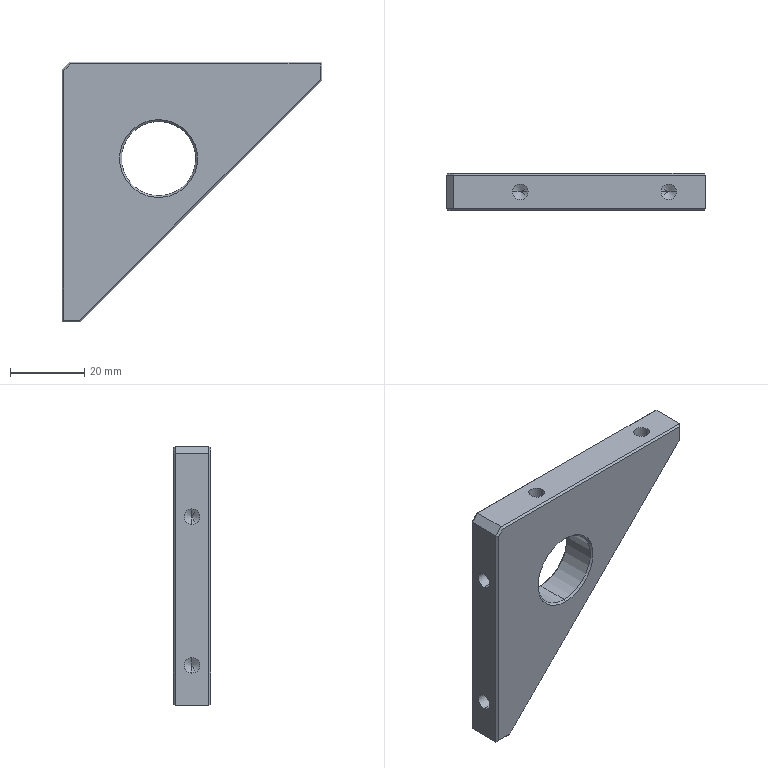Part | SolidWorks | features Chamfer 2, HoleWzd 2, Cut 1, Extrusion 1 | 1 solid | 42 faces | box 70 x 10 x 70 mm | volume 23927 mm3 | plane 20 | cone 12 | cylinder 10 | commonest cylinder face diameters 4.2 x8 20 x2
STEP:
#1=CARTESIAN_POINT('',(26.,4.5,-36.));
#2=VERTEX_POINT('',#1);
#3=CARTESIAN_POINT('',(26.,4.5,-16.));
#4=VERTEX_POINT('',#3);
#5=CARTESIAN_POINT('',(26.,4.5,-26.));
#6=DIRECTION('',(0.,1.,0.));
#7=DIRECTION('',(0.,0.,-1.));
#8=AXIS2_PLACEMENT_3D('',#5,#6,#7);
#9=CIRCLE('',#8,10.);
#10=EDGE_CURVE('',#2,#4,#9,.T.);
#11=ORIENTED_EDGE('',*,*,#10,.F.);
#12=CARTESIAN_POINT('',(26.,5.,-36.5));
#13=VERTEX_POINT('',#12);
#14=CARTESIAN_POINT('',(26.,5.,-36.5));
#15=DIRECTION('',(0.,0.7071,-0.7071));
#16=VECTOR('',#15,1000.);
#17=LINE('',#14,#16);
#18=EDGE_CURVE('',#2,#13,#17,.T.);
#19=ORIENTED_EDGE('',*,*,#18,.T.);
#20=CARTESIAN_POINT('',(26.,5.,-15.5));
#21=VERTEX_POINT('',#20);
#22=CARTESIAN_POINT('',(26.,5.,-26.));
#23=DIRECTION('',(0.,-1.,0.));
#24=DIRECTION('',(0.,0.,-1.));
#25=AXIS2_PLACEMENT_3D('',#22,#23,#24);
#26=CIRCLE('',#25,10.5);
#27=EDGE_CURVE('',#21,#13,#26,.T.);
#28=ORIENTED_EDGE('',*,*,#27,.F.);
#29=CARTESIAN_POINT('',(26.,5.,-15.5));
#30=DIRECTION('',(0.,0.7071,0.7071));
#31=VECTOR('',#30,1000.);
#32=LINE('',#29,#31);
#33=EDGE_CURVE('',#4,#21,#32,.T.);
#34=ORIENTED_EDGE('',*,*,#33,.F.);
#35=EDGE_LOOP('',(#11,#19,#28,#34));
#36=FACE_OUTER_BOUND('',#35,.T.);
#37=CARTESIAN_POINT('',(26.,5.,-26.));
#38=DIRECTION('',(0.,1.,0.));
#39=DIRECTION('',(0.,0.,1.));
#40=AXIS2_PLACEMENT_3D('',#37,#38,#39);
#41=CONICAL_SURFACE('',#40,10.5,0.7854);
#42=ADVANCED_FACE('',(#36),#41,.F.);
#43=CARTESIAN_POINT('',(26.,-4.5,-16.));
#44=VERTEX_POINT('',#43);
#45=CARTESIAN_POINT('',(26.,-4.5,-36.));
#46=VERTEX_POINT('',#45);
#47=CARTESIAN_POINT('',(26.,-4.5,-26.));
#48=DIRECTION('',(0.,-1.,0.));
#49=DIRECTION('',(0.,0.,-1.));
#50=AXIS2_PLACEMENT_3D('',#47,#48,#49);
#51=CIRCLE('',#50,10.);
#52=EDGE_CURVE('',#44,#46,#51,.T.);
#53=ORIENTED_EDGE('',*,*,#52,.F.);
#54=CARTESIAN_POINT('',(26.,-5.,-15.5));
#55=VERTEX_POINT('',#54);
#56=CARTESIAN_POINT('',(26.,-4.5,-16.));
#57=DIRECTION('',(0.,-0.7071,0.7071));
#58=VECTOR('',#57,1000.);
#59=LINE('',#56,#58);
#60=EDGE_CURVE('',#44,#55,#59,.T.);
#61=ORIENTED_EDGE('',*,*,#60,.T.);
#62=CARTESIAN_POINT('',(26.,-5.,-36.5));
#63=VERTEX_POINT('',#62);
#64=CARTESIAN_POINT('',(26.,-5.,-26.));
#65=DIRECTION('',(0.,1.,0.));
#66=DIRECTION('',(0.,0.,-1.));
#67=AXIS2_PLACEMENT_3D('',#64,#65,#66);
#68=CIRCLE('',#67,10.5);
#69=EDGE_CURVE('',#63,#55,#68,.T.);
#70=ORIENTED_EDGE('',*,*,#69,.F.);
#71=CARTESIAN_POINT('',(26.,-4.5,-36.));
#72=DIRECTION('',(0.,-0.7071,-0.7071));
#73=VECTOR('',#72,1000.);
#74=LINE('',#71,#73);
#75=EDGE_CURVE('',#46,#63,#74,.T.);
#76=ORIENTED_EDGE('',*,*,#75,.F.);
#77=EDGE_LOOP('',(#53,#61,#70,#76));
#78=FACE_OUTER_BOUND('',#77,.T.);
#79=CARTESIAN_POINT('',(26.,-4.5,-26.));
#80=DIRECTION('',(0.,-1.,0.));
#81=DIRECTION('',(0.,0.,-1.));
#82=AXIS2_PLACEMENT_3D('',#79,#80,#81);
#83=CONICAL_SURFACE('',#82,10.,0.7854);
#84=ADVANCED_FACE('',(#78),#83,.F.);
#85=ORIENTED_EDGE('',*,*,#10,.T.);
#86=CARTESIAN_POINT('',(26.,5.,-16.));
#87=DIRECTION('',(0.,-1.,0.));
#88=VECTOR('',#87,1000.);
#89=LINE('',#86,#88);
#90=EDGE_CURVE('',#4,#44,#89,.T.);
#91=ORIENTED_EDGE('',*,*,#90,.T.);
#92=ORIENTED_EDGE('',*,*,#52,.T.);
#93=CARTESIAN_POINT('',(26.,5.,-36.));
#94=DIRECTION('',(0.,-1.,0.));
#95=VECTOR('',#94,1000.);
#96=LINE('',#93,#95);
#97=EDGE_CURVE('',#2,#46,#96,.T.);
#98=ORIENTED_EDGE('',*,*,#97,.F.);
#99=EDGE_LOOP('',(#85,#91,#92,#98));
#100=FACE_OUTER_BOUND('',#99,.T.);
#101=CARTESIAN_POINT('',(26.,5.,-26.));
#102=DIRECTION('',(0.,-1.,0.));
#103=DIRECTION('',(0.,0.,-1.));
#104=AXIS2_PLACEMENT_3D('',#101,#102,#103);
#105=CYLINDRICAL_SURFACE('',#104,10.);
#106=ADVANCED_FACE('',(#100),#105,.F.);
#107=CARTESIAN_POINT('',(12.4,0.,-21.154));
#108=VERTEX_POINT('',#107);
#109=CARTESIAN_POINT('',(12.4,0.,-16.954));
#110=VERTEX_POINT('',#109);
#111=CARTESIAN_POINT('',(12.4,0.,-19.054));
#112=DIRECTION('',(-1.,0.,0.));
#113=DIRECTION('',(0.,0.,1.));
#114=AXIS2_PLACEMENT_3D('',#111,#112,#113);
#115=CIRCLE('',#114,2.1);
#116=EDGE_CURVE('',#108,#110,#115,.T.);
#117=ORIENTED_EDGE('',*,*,#116,.F.);
#118=CARTESIAN_POINT('',(0.,0.,-21.154));
#119=VERTEX_POINT('',#118);
#120=CARTESIAN_POINT('',(0.,0.,-21.154));
#121=DIRECTION('',(-1.,0.,0.));
#122=VECTOR('',#121,1000.);
#123=LINE('',#120,#122);
#124=EDGE_CURVE('',#108,#119,#123,.T.);
#125=ORIENTED_EDGE('',*,*,#124,.T.);
#126=CARTESIAN_POINT('',(0.,0.,-16.954));
#127=VERTEX_POINT('',#126);
#128=CARTESIAN_POINT('',(0.,0.,-19.054));
#129=DIRECTION('',(-1.,0.,0.));
#130=DIRECTION('',(0.,0.,1.));
#131=AXIS2_PLACEMENT_3D('',#128,#129,#130);
#132=CIRCLE('',#131,2.1);
#133=EDGE_CURVE('',#119,#127,#132,.T.);
#134=ORIENTED_EDGE('',*,*,#133,.T.);
#135=CARTESIAN_POINT('',(0.,0.,-16.954));
#136=DIRECTION('',(-1.,0.,0.));
#137=VECTOR('',#136,1000.);
#138=LINE('',#135,#137);
#139=EDGE_CURVE('',#110,#127,#138,.T.);
#140=ORIENTED_EDGE('',*,*,#139,.F.);
#141=EDGE_LOOP('',(#117,#125,#134,#140));
#142=FACE_OUTER_BOUND('',#141,.T.);
#143=CARTESIAN_POINT('',(0.,0.,-19.054));
#144=DIRECTION('',(-1.,0.,0.));
#145=DIRECTION('',(0.,0.,1.));
#146=AXIS2_PLACEMENT_3D('',#143,#144,#145);
#147=CYLINDRICAL_SURFACE('',#146,2.1);
#148=ADVANCED_FACE('',(#142),#147,.F.);
#149=CARTESIAN_POINT('',(13.662,0.,-19.054));
#150=VERTEX_POINT('',#149);
#151=CARTESIAN_POINT('',(12.4,0.,-16.954));
#152=DIRECTION('',(-0.515,0.,0.8572));
#153=VECTOR('',#152,1000.);
#154=LINE('',#151,#153);
#155=EDGE_CURVE('',#150,#110,#154,.T.);
#156=ORIENTED_EDGE('',*,*,#155,.F.);
#157=CARTESIAN_POINT('',(12.4,0.,-21.154));
#158=DIRECTION('',(-0.515,0.,-0.8572));
#159=VECTOR('',#158,1000.);
#160=LINE('',#157,#159);
#161=EDGE_CURVE('',#150,#108,#160,.T.);
#162=ORIENTED_EDGE('',*,*,#161,.T.);
#163=ORIENTED_EDGE('',*,*,#116,.T.);
#164=EDGE_LOOP('',(#156,#162,#163));
#165=FACE_OUTER_BOUND('',#164,.T.);
#166=CARTESIAN_POINT('',(12.4,0.,-19.054));
#167=DIRECTION('',(-1.,0.,0.));
#168=DIRECTION('',(0.,0.,1.));
#169=AXIS2_PLACEMENT_3D('',#166,#167,#168);
#170=CONICAL_SURFACE('',#169,2.1,1.03);
#171=ADVANCED_FACE('',(#165),#170,.F.);
#172=CARTESIAN_POINT('',(12.4,0.,-61.154));
#173=VERTEX_POINT('',#172);
#174=CARTESIAN_POINT('',(12.4,0.,-56.954));
#175=VERTEX_POINT('',#174);
#176=CARTESIAN_POINT('',(12.4,0.,-59.054));
#177=DIRECTION('',(-1.,0.,0.));
#178=DIRECTION('',(0.,0.,1.));
#179=AXIS2_PLACEMENT_3D('',#176,#177,#178);
#180=CIRCLE('',#179,2.1);
#181=EDGE_CURVE('',#173,#175,#180,.T.);
#182=ORIENTED_EDGE('',*,*,#181,.F.);
#183=CARTESIAN_POINT('',(0.,0.,-61.154));
#184=VERTEX_POINT('',#183);
#185=CARTESIAN_POINT('',(0.,0.,-61.154));
#186=DIRECTION('',(-1.,0.,0.));
#187=VECTOR('',#186,1000.);
#188=LINE('',#185,#187);
#189=EDGE_CURVE('',#173,#184,#188,.T.);
#190=ORIENTED_EDGE('',*,*,#189,.T.);
#191=CARTESIAN_POINT('',(0.,0.,-56.954));
#192=VERTEX_POINT('',#191);
#193=CARTESIAN_POINT('',(0.,0.,-59.054));
#194=DIRECTION('',(-1.,0.,0.));
#195=DIRECTION('',(0.,0.,1.));
#196=AXIS2_PLACEMENT_3D('',#193,#194,#195);
#197=CIRCLE('',#196,2.1);
#198=EDGE_CURVE('',#184,#192,#197,.T.);
#199=ORIENTED_EDGE('',*,*,#198,.T.);
#200=CARTESIAN_POINT('',(0.,0.,-56.954));
#201=DIRECTION('',(-1.,0.,0.));
#202=VECTOR('',#201,1000.);
#203=LINE('',#200,#202);
#204=EDGE_CURVE('',#175,#192,#203,.T.);
#205=ORIENTED_EDGE('',*,*,#204,.F.);
#206=EDGE_LOOP('',(#182,#190,#199,#205));
#207=FACE_OUTER_BOUND('',#206,.T.);
#208=CARTESIAN_POINT('',(0.,0.,-59.054));
#209=DIRECTION('',(-1.,0.,0.));
#210=DIRECTION('',(0.,0.,1.));
#211=AXIS2_PLACEMENT_3D('',#208,#209,#210);
#212=CYLINDRICAL_SURFACE('',#211,2.1);
#213=ADVANCED_FACE('',(#207),#212,.F.);
#214=CARTESIAN_POINT('',(13.662,0.,-59.054));
#215=VERTEX_POINT('',#214);
#216=CARTESIAN_POINT('',(12.4,0.,-56.954));
#217=DIRECTION('',(-0.515,0.,0.8572));
#218=VECTOR('',#217,1000.);
#219=LINE('',#216,#218);
#220=EDGE_CURVE('',#215,#175,#219,.T.);
#221=ORIENTED_EDGE('',*,*,#220,.F.);
#222=CARTESIAN_POINT('',(12.4,0.,-61.154));
#223=DIRECTION('',(-0.515,0.,-0.8572));
#224=VECTOR('',#223,1000.);
#225=LINE('',#222,#224);
#226=EDGE_CURVE('',#215,#173,#225,.T.);
#227=ORIENTED_EDGE('',*,*,#226,.T.);
#228=ORIENTED_EDGE('',*,*,#181,.T.);
#229=EDGE_LOOP('',(#221,#227,#228));
#230=FACE_OUTER_BOUND('',#229,.T.);
#231=CARTESIAN_POINT('',(12.4,0.,-59.054));
#232=DIRECTION('',(-1.,0.,0.));
#233=DIRECTION('',(0.,0.,1.));
#234=AXIS2_PLACEMENT_3D('',#231,#232,#233);
#235=CONICAL_SURFACE('',#234,2.1,1.03);
#236=ADVANCED_FACE('',(#230),#235,.F.);
#237=CARTESIAN_POINT('',(57.9,0.,-12.4));
#238=VERTEX_POINT('',#237);
#239=CARTESIAN_POINT('',(62.1,0.,-12.4));
#240=VERTEX_POINT('',#239);
#241=CARTESIAN_POINT('',(60.,0.,-12.4));
#242=DIRECTION('',(0.,0.,1.));
#243=DIRECTION('',(1.,0.,0.));
#244=AXIS2_PLACEMENT_3D('',#241,#242,#243);
#245=CIRCLE('',#244,2.1);
#246=EDGE_CURVE('',#238,#240,#245,.T.);
#247=ORIENTED_EDGE('',*,*,#246,.F.);
#248=CARTESIAN_POINT('',(57.9,0.,0.));
#249=VERTEX_POINT('',#248);
#250=CARTESIAN_POINT('',(57.9,0.,0.));
#251=DIRECTION('',(0.,0.,1.));
#252=VECTOR('',#251,1000.);
#253=LINE('',#250,#252);
#254=EDGE_CURVE('',#238,#249,#253,.T.);
#255=ORIENTED_EDGE('',*,*,#254,.T.);
#256=CARTESIAN_POINT('',(62.1,0.,0.));
#257=VERTEX_POINT('',#256);
#258=CARTESIAN_POINT('',(60.,0.,0.));
#259=DIRECTION('',(0.,0.,1.));
#260=DIRECTION('',(1.,0.,0.));
#261=AXIS2_PLACEMENT_3D('',#258,#259,#260);
#262=CIRCLE('',#261,2.1);
#263=EDGE_CURVE('',#249,#257,#262,.T.);
#264=ORIENTED_EDGE('',*,*,#263,.T.);
#265=CARTESIAN_POINT('',(62.1,0.,0.));
#266=DIRECTION('',(0.,0.,1.));
#267=VECTOR('',#266,1000.);
#268=LINE('',#265,#267);
#269=EDGE_CURVE('',#240,#257,#268,.T.);
#270=ORIENTED_EDGE('',*,*,#269,.F.);
#271=EDGE_LOOP('',(#247,#255,#264,#270));
#272=FACE_OUTER_BOUND('',#271,.T.);
#273=CARTESIAN_POINT('',(60.,0.,0.));
#274=DIRECTION('',(0.,0.,1.));
#275=DIRECTION('',(1.,0.,0.));
#276=AXIS2_PLACEMENT_3D('',#273,#274,#275);
#277=CYLINDRICAL_SURFACE('',#276,2.1);
#278=ADVANCED_FACE('',(#272),#277,.F.);
#279=CARTESIAN_POINT('',(60.,0.,-13.662));
#280=VERTEX_POINT('',#279);
#281=CARTESIAN_POINT('',(62.1,0.,-12.4));
#282=DIRECTION('',(0.8572,0.,0.515));
#283=VECTOR('',#282,1000.);
#284=LINE('',#281,#283);
#285=EDGE_CURVE('',#280,#240,#284,.T.);
#286=ORIENTED_EDGE('',*,*,#285,.F.);
#287=CARTESIAN_POINT('',(57.9,0.,-12.4));
#288=DIRECTION('',(-0.8572,0.,0.515));
#289=VECTOR('',#288,1000.);
#290=LINE('',#287,#289);
#291=EDGE_CURVE('',#280,#238,#290,.T.);
#292=ORIENTED_EDGE('',*,*,#291,.T.);
#293=ORIENTED_EDGE('',*,*,#246,.T.);
#294=EDGE_LOOP('',(#286,#292,#293));
#295=FACE_OUTER_BOUND('',#294,.T.);
#296=CARTESIAN_POINT('',(60.,0.,-12.4));
#297=DIRECTION('',(0.,0.,1.));
#298=DIRECTION('',(1.,0.,0.));
#299=AXIS2_PLACEMENT_3D('',#296,#297,#298);
#300=CONICAL_SURFACE('',#299,2.1,1.03);
#301=ADVANCED_FACE('',(#295),#300,.F.);
#302=CARTESIAN_POINT('',(17.9,0.,-12.4));
#303=VERTEX_POINT('',#302);
#304=CARTESIAN_POINT('',(22.1,0.,-12.4));
#305=VERTEX_POINT('',#304);
#306=CARTESIAN_POINT('',(20.,0.,-12.4));
#307=DIRECTION('',(0.,0.,1.));
#308=DIRECTION('',(1.,0.,0.));
#309=AXIS2_PLACEMENT_3D('',#306,#307,#308);
#310=CIRCLE('',#309,2.1);
#311=EDGE_CURVE('',#303,#305,#310,.T.);
#312=ORIENTED_EDGE('',*,*,#311,.F.);
#313=CARTESIAN_POINT('',(17.9,0.,0.));
#314=VERTEX_POINT('',#313);
#315=CARTESIAN_POINT('',(17.9,0.,0.));
#316=DIRECTION('',(0.,0.,1.));
#317=VECTOR('',#316,1000.);
#318=LINE('',#315,#317);
#319=EDGE_CURVE('',#303,#314,#318,.T.);
#320=ORIENTED_EDGE('',*,*,#319,.T.);
#321=CARTESIAN_POINT('',(22.1,0.,0.));
#322=VERTEX_POINT('',#321);
#323=CARTESIAN_POINT('',(20.,0.,0.));
#324=DIRECTION('',(0.,0.,1.));
#325=DIRECTION('',(1.,0.,0.));
#326=AXIS2_PLACEMENT_3D('',#323,#324,#325);
#327=CIRCLE('',#326,2.1);
#328=EDGE_CURVE('',#314,#322,#327,.T.);
#329=ORIENTED_EDGE('',*,*,#328,.T.);
#330=CARTESIAN_POINT('',(22.1,0.,0.));
#331=DIRECTION('',(0.,0.,1.));
#332=VECTOR('',#331,1000.);
#333=LINE('',#330,#332);
#334=EDGE_CURVE('',#305,#322,#333,.T.);
#335=ORIENTED_EDGE('',*,*,#334,.F.);
#336=EDGE_LOOP('',(#312,#320,#329,#335));
#337=FACE_OUTER_BOUND('',#336,.T.);
#338=CARTESIAN_POINT('',(20.,0.,0.));
#339=DIRECTION('',(0.,0.,1.));
#340=DIRECTION('',(1.,0.,0.));
#341=AXIS2_PLACEMENT_3D('',#338,#339,#340);
#342=CYLINDRICAL_SURFACE('',#341,2.1);
#343=ADVANCED_FACE('',(#337),#342,.F.);
#344=CARTESIAN_POINT('',(20.,0.,-13.662));
#345=VERTEX_POINT('',#344);
#346=CARTESIAN_POINT('',(22.1,0.,-12.4));
#347=DIRECTION('',(0.8572,0.,0.515));
#348=VECTOR('',#347,1000.);
#349=LINE('',#346,#348);
#350=EDGE_CURVE('',#345,#305,#349,.T.);
#351=ORIENTED_EDGE('',*,*,#350,.F.);
#352=CARTESIAN_POINT('',(17.9,0.,-12.4));
#353=DIRECTION('',(-0.8572,0.,0.515));
#354=VECTOR('',#353,1000.);
#355=LINE('',#352,#354);
#356=EDGE_CURVE('',#345,#303,#355,.T.);
#357=ORIENTED_EDGE('',*,*,#356,.T.);
#358=ORIENTED_EDGE('',*,*,#311,.T.);
#359=EDGE_LOOP('',(#351,#357,#358));
#360=FACE_OUTER_BOUND('',#359,.T.);
#361=CARTESIAN_POINT('',(20.,0.,-12.4));
#362=DIRECTION('',(0.,0.,1.));
#363=DIRECTION('',(1.,0.,0.));
#364=AXIS2_PLACEMENT_3D('',#361,#362,#363);
#365=CONICAL_SURFACE('',#364,2.1,1.03);
#366=ADVANCED_FACE('',(#360),#365,.F.);
#367=CARTESIAN_POINT('',(60.,0.,0.));
#368=DIRECTION('',(0.,0.,1.));
#369=DIRECTION('',(1.,0.,0.));
#370=AXIS2_PLACEMENT_3D('',#367,#368,#369);
#371=CIRCLE('',#370,2.1);
#372=EDGE_CURVE('',#257,#249,#371,.T.);
#373=ORIENTED_EDGE('',*,*,#372,.F.);
#374=ORIENTED_EDGE('',*,*,#263,.F.);
#375=EDGE_LOOP('',(#373,#374));
#376=FACE_BOUND('',#375,.T.);
#377=CARTESIAN_POINT('',(20.,0.,0.));
#378=DIRECTION('',(0.,0.,1.));
#379=DIRECTION('',(1.,0.,0.));
#380=AXIS2_PLACEMENT_3D('',#377,#378,#379);
#381=CIRCLE('',#380,2.1);
#382=EDGE_CURVE('',#322,#314,#381,.T.);
#383=ORIENTED_EDGE('',*,*,#382,.F.);
#384=ORIENTED_EDGE('',*,*,#328,.F.);
#385=EDGE_LOOP('',(#383,#384));
#386=FACE_BOUND('',#385,.T.);
#387=CARTESIAN_POINT('',(2.,4.5,0.));
#388=VERTEX_POINT('',#387);
#389=CARTESIAN_POINT('',(2.,-4.5,0.));
#390=VERTEX_POINT('',#389);
#391=CARTESIAN_POINT('',(2.,5.,0.));
#392=DIRECTION('',(0.,-1.,0.));
#393=VECTOR('',#392,1000.);
#394=LINE('',#391,#393);
#395=EDGE_CURVE('',#388,#390,#394,.T.);
#396=ORIENTED_EDGE('',*,*,#395,.T.);
#397=CARTESIAN_POINT('',(70.,-4.5,0.));
#398=VERTEX_POINT('',#397);
#399=CARTESIAN_POINT('',(70.,-4.5,0.));
#400=DIRECTION('',(1.,0.,0.));
#401=VECTOR('',#400,1000.);
#402=LINE('',#399,#401);
#403=EDGE_CURVE('',#390,#398,#402,.T.);
#404=ORIENTED_EDGE('',*,*,#403,.T.);
#405=CARTESIAN_POINT('',(70.,4.5,0.));
#406=VERTEX_POINT('',#405);
#407=CARTESIAN_POINT('',(70.,5.,0.));
#408=DIRECTION('',(0.,-1.,0.));
#409=VECTOR('',#408,1000.);
#410=LINE('',#407,#409);
#411=EDGE_CURVE('',#406,#398,#410,.T.);
#412=ORIENTED_EDGE('',*,*,#411,.F.);
#413=CARTESIAN_POINT('',(70.,4.5,0.));
#414=DIRECTION('',(-1.,0.,0.));
#415=VECTOR('',#414,1000.);
#416=LINE('',#413,#415);
#417=EDGE_CURVE('',#406,#388,#416,.T.);
#418=ORIENTED_EDGE('',*,*,#417,.T.);
#419=EDGE_LOOP('',(#396,#404,#412,#418));
#420=FACE_OUTER_BOUND('',#419,.T.);
#421=CARTESIAN_POINT('',(70.,5.,0.));
#422=DIRECTION('',(0.,0.,-1.));
#423=DIRECTION('',(-1.,0.,0.));
#424=AXIS2_PLACEMENT_3D('',#421,#422,#423);
#425=PLANE('',#424);
#426=ADVANCED_FACE('',(#376,#386,#420),#425,.F.);
#427=ORIENTED_EDGE('',*,*,#411,.T.);
#428=CARTESIAN_POINT('',(70.,-4.5,-5.));
#429=VERTEX_POINT('',#428);
#430=CARTESIAN_POINT('',(70.,-4.5,-5.));
#431=DIRECTION('',(0.,0.,-1.));
#432=VECTOR('',#431,1000.);
#433=LINE('',#430,#432);
#434=EDGE_CURVE('',#398,#429,#433,.T.);
#435=ORIENTED_EDGE('',*,*,#434,.T.);
#436=CARTESIAN_POINT('',(70.,4.5,-5.));
#437=VERTEX_POINT('',#436);
#438=CARTESIAN_POINT('',(70.,5.,-5.));
#439=DIRECTION('',(0.,-1.,0.));
#440=VECTOR('',#439,1000.);
#441=LINE('',#438,#440);
#442=EDGE_CURVE('',#437,#429,#441,.T.);
#443=ORIENTED_EDGE('',*,*,#442,.F.);
#444=CARTESIAN_POINT('',(70.,4.5,-5.));
#445=DIRECTION('',(0.,0.,1.));
#446=VECTOR('',#445,1000.);
#447=LINE('',#444,#446);
#448=EDGE_CURVE('',#437,#406,#447,.T.);
#449=ORIENTED_EDGE('',*,*,#448,.T.);
#450=EDGE_LOOP('',(#427,#435,#443,#449));
#451=FACE_OUTER_BOUND('',#450,.T.);
#452=CARTESIAN_POINT('',(70.,5.,-5.));
#453=DIRECTION('',(-1.,0.,0.));
#454=DIRECTION('',(0.,0.,1.));
#455=AXIS2_PLACEMENT_3D('',#452,#453,#454);
#456=PLANE('',#455);
#457=ADVANCED_FACE('',(#451),#456,.F.);
#458=ORIENTED_EDGE('',*,*,#442,.T.);
#459=CARTESIAN_POINT('',(5.,-4.5,-70.));
#460=VERTEX_POINT('',#459);
#461=CARTESIAN_POINT('',(5.,-4.5,-70.));
#462=DIRECTION('',(-0.7071,0.,-0.7071));
#463=VECTOR('',#462,1000.);
#464=LINE('',#461,#463);
#465=EDGE_CURVE('',#429,#460,#464,.T.);
#466=ORIENTED_EDGE('',*,*,#465,.T.);
#467=CARTESIAN_POINT('',(5.,4.5,-70.));
#468=VERTEX_POINT('',#467);
#469=CARTESIAN_POINT('',(5.,5.,-70.));
#470=DIRECTION('',(0.,-1.,0.));
#471=VECTOR('',#470,1000.);
#472=LINE('',#469,#471);
#473=EDGE_CURVE('',#468,#460,#472,.T.);
#474=ORIENTED_EDGE('',*,*,#473,.F.);
#475=CARTESIAN_POINT('',(5.,4.5,-70.));
#476=DIRECTION('',(0.7071,0.,0.7071));
#477=VECTOR('',#476,1000.);
#478=LINE('',#475,#477);
#479=EDGE_CURVE('',#468,#437,#478,.T.);
#480=ORIENTED_EDGE('',*,*,#479,.T.);
#481=EDGE_LOOP('',(#458,#466,#474,#480));
#482=FACE_OUTER_BOUND('',#481,.T.);
#483=CARTESIAN_POINT('',(5.,5.,-70.));
#484=DIRECTION('',(-0.7071,0.,0.7071));
#485=DIRECTION('',(0.7071,0.,0.7071));
#486=AXIS2_PLACEMENT_3D('',#483,#484,#485);
#487=PLANE('',#486);
#488=ADVANCED_FACE('',(#482),#487,.F.);
#489=ORIENTED_EDGE('',*,*,#473,.T.);
#490=CARTESIAN_POINT('',(0.,-4.5,-70.));
#491=VERTEX_POINT('',#490);
#492=CARTESIAN_POINT('',(0.,-4.5,-70.));
#493=DIRECTION('',(-1.,0.,0.));
#494=VECTOR('',#493,1000.);
#495=LINE('',#492,#494);
#496=EDGE_CURVE('',#460,#491,#495,.T.);
#497=ORIENTED_EDGE('',*,*,#496,.T.);
#498=CARTESIAN_POINT('',(0.,4.5,-70.));
#499=VERTEX_POINT('',#498);
#500=CARTESIAN_POINT('',(0.,5.,-70.));
#501=DIRECTION('',(0.,-1.,0.));
#502=VECTOR('',#501,1000.);
#503=LINE('',#500,#502);
#504=EDGE_CURVE('',#499,#491,#503,.T.);
#505=ORIENTED_EDGE('',*,*,#504,.F.);
#506=CARTESIAN_POINT('',(0.,4.5,-70.));
#507=DIRECTION('',(1.,0.,0.));
#508=VECTOR('',#507,1000.);
#509=LINE('',#506,#508);
#510=EDGE_CURVE('',#499,#468,#509,.T.);
#511=ORIENTED_EDGE('',*,*,#510,.T.);
#512=EDGE_LOOP('',(#489,#497,#505,#511));
#513=FACE_OUTER_BOUND('',#512,.T.);
#514=CARTESIAN_POINT('',(0.,5.,-70.));
#515=DIRECTION('',(0.,0.,1.));
#516=DIRECTION('',(1.,0.,0.));
#517=AXIS2_PLACEMENT_3D('',#514,#515,#516);
#518=PLANE('',#517);
#519=ADVANCED_FACE('',(#513),#518,.F.);
#520=CARTESIAN_POINT('',(0.,0.,-19.054));
#521=DIRECTION('',(-1.,0.,0.));
#522=DIRECTION('',(0.,0.,1.));
#523=AXIS2_PLACEMENT_3D('',#520,#521,#522);
#524=CIRCLE('',#523,2.1);
#525=EDGE_CURVE('',#127,#119,#524,.T.);
#526=ORIENTED_EDGE('',*,*,#525,.F.);
#527=ORIENTED_EDGE('',*,*,#133,.F.);
#528=EDGE_LOOP('',(#526,#527));
#529=FACE_BOUND('',#528,.T.);
#530=CARTESIAN_POINT('',(0.,0.,-59.054));
#531=DIRECTION('',(-1.,0.,0.));
#532=DIRECTION('',(0.,0.,1.));
#533=AXIS2_PLACEMENT_3D('',#530,#531,#532);
#534=CIRCLE('',#533,2.1);
#535=EDGE_CURVE('',#192,#184,#534,.T.);
#536=ORIENTED_EDGE('',*,*,#535,.F.);
#537=ORIENTED_EDGE('',*,*,#198,.F.);
#538=EDGE_LOOP('',(#536,#537));
#539=FACE_BOUND('',#538,.T.);
#540=ORIENTED_EDGE('',*,*,#504,.T.);
#541=CARTESIAN_POINT('',(0.,-4.5,-2.));
#542=VERTEX_POINT('',#541);
#543=CARTESIAN_POINT('',(0.,-4.5,-2.));
#544=DIRECTION('',(0.,0.,1.));
#545=VECTOR('',#544,1000.);
#546=LINE('',#543,#545);
#547=EDGE_CURVE('',#491,#542,#546,.T.);
#548=ORIENTED_EDGE('',*,*,#547,.T.);
#549=CARTESIAN_POINT('',(0.,4.5,-2.));
#550=VERTEX_POINT('',#549);
#551=CARTESIAN_POINT('',(0.,5.,-2.));
#552=DIRECTION('',(0.,1.,0.));
#553=VECTOR('',#552,1000.);
#554=LINE('',#551,#553);
#555=EDGE_CURVE('',#542,#550,#554,.T.);
#556=ORIENTED_EDGE('',*,*,#555,.T.);
#557=CARTESIAN_POINT('',(0.,4.5,0.));
#558=DIRECTION('',(0.,0.,-1.));
#559=VECTOR('',#558,1000.);
#560=LINE('',#557,#559);
#561=EDGE_CURVE('',#550,#499,#560,.T.);
#562=ORIENTED_EDGE('',*,*,#561,.T.);
#563=EDGE_LOOP('',(#540,#548,#556,#562));
#564=FACE_OUTER_BOUND('',#563,.T.);
#565=CARTESIAN_POINT('',(0.,5.,0.));
#566=DIRECTION('',(1.,0.,0.));
#567=DIRECTION('',(0.,0.,-1.));
#568=AXIS2_PLACEMENT_3D('',#565,#566,#567);
#569=PLANE('',#568);
#570=ADVANCED_FACE('',(#529,#539,#564),#569,.F.);
#571=CARTESIAN_POINT('',(69.5,5.,-4.793));
#572=VERTEX_POINT('',#571);
#573=CARTESIAN_POINT('',(4.793,5.,-69.5));
#574=VERTEX_POINT('',#573);
#575=CARTESIAN_POINT('',(37.146,5.,-37.146));
#576=DIRECTION('',(-0.7071,0.,-0.7071));
#577=VECTOR('',#576,1000.);
#578=LINE('',#575,#577);
#579=EDGE_CURVE('',#572,#574,#578,.T.);
#580=ORIENTED_EDGE('',*,*,#579,.T.);
#581=CARTESIAN_POINT('',(0.5,5.,-69.5));
#582=VERTEX_POINT('',#581);
#583=CARTESIAN_POINT('',(0.,5.,-69.5));
#584=DIRECTION('',(-1.,0.,0.));
#585=VECTOR('',#584,1000.);
#586=LINE('',#583,#585);
#587=EDGE_CURVE('',#574,#582,#586,.T.);
#588=ORIENTED_EDGE('',*,*,#587,.T.);
#589=CARTESIAN_POINT('',(0.5,5.,-2.207));
#590=VERTEX_POINT('',#589);
#591=CARTESIAN_POINT('',(0.5,5.,0.));
#592=DIRECTION('',(0.,0.,1.));
#593=VECTOR('',#592,1000.);
#594=LINE('',#591,#593);
#595=EDGE_CURVE('',#582,#590,#594,.T.);
#596=ORIENTED_EDGE('',*,*,#595,.T.);
#597=CARTESIAN_POINT('',(2.207,5.,-0.5));
#598=VERTEX_POINT('',#597);
#599=CARTESIAN_POINT('',(2.354,5.,-0.3536));
#600=DIRECTION('',(0.7071,0.,0.7071));
#601=VECTOR('',#600,1000.);
#602=LINE('',#599,#601);
#603=EDGE_CURVE('',#590,#598,#602,.T.);
#604=ORIENTED_EDGE('',*,*,#603,.T.);
#605=CARTESIAN_POINT('',(69.5,5.,-0.5));
#606=VERTEX_POINT('',#605);
#607=CARTESIAN_POINT('',(0.,5.,-0.5));
#608=DIRECTION('',(1.,0.,0.));
#609=VECTOR('',#608,1000.);
#610=LINE('',#607,#609);
#611=EDGE_CURVE('',#598,#606,#610,.T.);
#612=ORIENTED_EDGE('',*,*,#611,.T.);
#613=CARTESIAN_POINT('',(69.5,5.,0.));
#614=DIRECTION('',(0.,0.,-1.));
#615=VECTOR('',#614,1000.);
#616=LINE('',#613,#615);
#617=EDGE_CURVE('',#606,#572,#616,.T.);
#618=ORIENTED_EDGE('',*,*,#617,.T.);
#619=EDGE_LOOP('',(#580,#588,#596,#604,#612,#618));
#620=FACE_OUTER_BOUND('',#619,.T.);
#621=ORIENTED_EDGE('',*,*,#27,.T.);
#622=CARTESIAN_POINT('',(26.,5.,-26.));
#623=DIRECTION('',(0.,-1.,0.));
#624=DIRECTION('',(0.,0.,-1.));
#625=AXIS2_PLACEMENT_3D('',#622,#623,#624);
#626=CIRCLE('',#625,10.5);
#627=EDGE_CURVE('',#13,#21,#626,.T.);
#628=ORIENTED_EDGE('',*,*,#627,.T.);
#629=EDGE_LOOP('',(#621,#628));
#630=FACE_BOUND('',#629,.T.);
#631=CARTESIAN_POINT('',(0.,5.,0.));
#632=DIRECTION('',(0.,-1.,0.));
#633=DIRECTION('',(0.,0.,-1.));
#634=AXIS2_PLACEMENT_3D('',#631,#632,#633);
#635=PLANE('',#634);
#636=ADVANCED_FACE('',(#620,#630),#635,.F.);
#637=CARTESIAN_POINT('',(4.793,-5.,-69.5));
#638=VERTEX_POINT('',#637);
#639=CARTESIAN_POINT('',(69.5,-5.,-4.793));
#640=VERTEX_POINT('',#639);
#641=CARTESIAN_POINT('',(69.646,-5.,-4.646));
#642=DIRECTION('',(0.7071,0.,0.7071));
#643=VECTOR('',#642,1000.);
#644=LINE('',#641,#643);
#645=EDGE_CURVE('',#638,#640,#644,.T.);
#646=ORIENTED_EDGE('',*,*,#645,.T.);
#647=CARTESIAN_POINT('',(69.5,-5.,-0.5));
#648=VERTEX_POINT('',#647);
#649=CARTESIAN_POINT('',(69.5,-5.,0.));
#650=DIRECTION('',(0.,0.,1.));
#651=VECTOR('',#650,1000.);
#652=LINE('',#649,#651);
#653=EDGE_CURVE('',#640,#648,#652,.T.);
#654=ORIENTED_EDGE('',*,*,#653,.T.);
#655=CARTESIAN_POINT('',(2.207,-5.,-0.5));
#656=VERTEX_POINT('',#655);
#657=CARTESIAN_POINT('',(2.,-5.,-0.5));
#658=DIRECTION('',(-1.,0.,0.));
#659=VECTOR('',#658,1000.);
#660=LINE('',#657,#659);
#661=EDGE_CURVE('',#648,#656,#660,.T.);
#662=ORIENTED_EDGE('',*,*,#661,.T.);
#663=CARTESIAN_POINT('',(0.5,-5.,-2.207));
#664=VERTEX_POINT('',#663);
#665=CARTESIAN_POINT('',(1.354,-5.,-1.354));
#666=DIRECTION('',(-0.7071,0.,-0.7071));
#667=VECTOR('',#666,1000.);
#668=LINE('',#665,#667);
#669=EDGE_CURVE('',#656,#664,#668,.T.);
#670=ORIENTED_EDGE('',*,*,#669,.T.);
#671=CARTESIAN_POINT('',(0.5,-5.,-69.5));
#672=VERTEX_POINT('',#671);
#673=CARTESIAN_POINT('',(0.5,-5.,-70.));
#674=DIRECTION('',(0.,0.,-1.));
#675=VECTOR('',#674,1000.);
#676=LINE('',#673,#675);
#677=EDGE_CURVE('',#664,#672,#676,.T.);
#678=ORIENTED_EDGE('',*,*,#677,.T.);
#679=CARTESIAN_POINT('',(5.,-5.,-69.5));
#680=DIRECTION('',(1.,0.,0.));
#681=VECTOR('',#680,1000.);
#682=LINE('',#679,#681);
#683=EDGE_CURVE('',#672,#638,#682,.T.);
#684=ORIENTED_EDGE('',*,*,#683,.T.);
#685=EDGE_LOOP('',(#646,#654,#662,#670,#678,#684));
#686=FACE_OUTER_BOUND('',#685,.T.);
#687=ORIENTED_EDGE('',*,*,#69,.T.);
#688=CARTESIAN_POINT('',(26.,-5.,-26.));
#689=DIRECTION('',(0.,1.,0.));
#690=DIRECTION('',(0.,0.,-1.));
#691=AXIS2_PLACEMENT_3D('',#688,#689,#690);
#692=CIRCLE('',#691,10.5);
#693=EDGE_CURVE('',#55,#63,#692,.T.);
#694=ORIENTED_EDGE('',*,*,#693,.T.);
#695=EDGE_LOOP('',(#687,#694));
#696=FACE_BOUND('',#695,.T.);
#697=CARTESIAN_POINT('',(0.,-5.,0.));
#698=DIRECTION('',(0.,-1.,0.));
#699=DIRECTION('',(0.,0.,-1.));
#700=AXIS2_PLACEMENT_3D('',#697,#698,#699);
#701=PLANE('',#700);
#702=ADVANCED_FACE('',(#686,#696),#701,.T.);
#703=ORIENTED_EDGE('',*,*,#555,.F.);
#704=CARTESIAN_POINT('',(2.,-4.5,0.));
#705=DIRECTION('',(0.7071,0.,0.7071));
#706=VECTOR('',#705,1000.);
#707=LINE('',#704,#706);
#708=EDGE_CURVE('',#542,#390,#707,.T.);
#709=ORIENTED_EDGE('',*,*,#708,.T.);
#710=ORIENTED_EDGE('',*,*,#395,.F.);
#711=CARTESIAN_POINT('',(0.,4.5,-2.));
#712=DIRECTION('',(-0.7071,0.,-0.7071));
#713=VECTOR('',#712,1000.);
#714=LINE('',#711,#713);
#715=EDGE_CURVE('',#388,#550,#714,.T.);
#716=ORIENTED_EDGE('',*,*,#715,.T.);
#717=EDGE_LOOP('',(#703,#709,#710,#716));
#718=FACE_OUTER_BOUND('',#717,.T.);
#719=CARTESIAN_POINT('',(2.,5.,0.));
#720=DIRECTION('',(0.7071,0.,-0.7071));
#721=DIRECTION('',(0.,-1.,0.));
#722=AXIS2_PLACEMENT_3D('',#719,#720,#721);
#723=PLANE('',#722);
#724=ADVANCED_FACE('',(#718),#723,.F.);
#725=ORIENTED_EDGE('',*,*,#356,.F.);
#726=ORIENTED_EDGE('',*,*,#350,.T.);
#727=CARTESIAN_POINT('',(20.,0.,-12.4));
#728=DIRECTION('',(0.,0.,1.));
#729=DIRECTION('',(1.,0.,0.));
#730=AXIS2_PLACEMENT_3D('',#727,#728,#729);
#731=CIRCLE('',#730,2.1);
#732=EDGE_CURVE('',#305,#303,#731,.T.);
#733=ORIENTED_EDGE('',*,*,#732,.T.);
#734=EDGE_LOOP('',(#725,#726,#733));
#735=FACE_OUTER_BOUND('',#734,.T.);
#736=CARTESIAN_POINT('',(20.,0.,-12.4));
#737=DIRECTION('',(0.,0.,1.));
#738=DIRECTION('',(1.,0.,0.));
#739=AXIS2_PLACEMENT_3D('',#736,#737,#738);
#740=CONICAL_SURFACE('',#739,2.1,1.03);
#741=ADVANCED_FACE('',(#735),#740,.F.);
#742=ORIENTED_EDGE('',*,*,#319,.F.);
#743=ORIENTED_EDGE('',*,*,#732,.F.);
#744=ORIENTED_EDGE('',*,*,#334,.T.);
#745=ORIENTED_EDGE('',*,*,#382,.T.);
#746=EDGE_LOOP('',(#742,#743,#744,#745));
#747=FACE_OUTER_BOUND('',#746,.T.);
#748=CARTESIAN_POINT('',(20.,0.,0.));
#749=DIRECTION('',(0.,0.,1.));
#750=DIRECTION('',(1.,0.,0.));
#751=AXIS2_PLACEMENT_3D('',#748,#749,#750);
#752=CYLINDRICAL_SURFACE('',#751,2.1);
#753=ADVANCED_FACE('',(#747),#752,.F.);
#754=ORIENTED_EDGE('',*,*,#291,.F.);
#755=ORIENTED_EDGE('',*,*,#285,.T.);
#756=CARTESIAN_POINT('',(60.,0.,-12.4));
#757=DIRECTION('',(0.,0.,1.));
#758=DIRECTION('',(1.,0.,0.));
#759=AXIS2_PLACEMENT_3D('',#756,#757,#758);
#760=CIRCLE('',#759,2.1);
#761=EDGE_CURVE('',#240,#238,#760,.T.);
#762=ORIENTED_EDGE('',*,*,#761,.T.);
#763=EDGE_LOOP('',(#754,#755,#762));
#764=FACE_OUTER_BOUND('',#763,.T.);
#765=CARTESIAN_POINT('',(60.,0.,-12.4));
#766=DIRECTION('',(0.,0.,1.));
#767=DIRECTION('',(1.,0.,0.));
#768=AXIS2_PLACEMENT_3D('',#765,#766,#767);
#769=CONICAL_SURFACE('',#768,2.1,1.03);
#770=ADVANCED_FACE('',(#764),#769,.F.);
#771=ORIENTED_EDGE('',*,*,#254,.F.);
#772=ORIENTED_EDGE('',*,*,#761,.F.);
#773=ORIENTED_EDGE('',*,*,#269,.T.);
#774=ORIENTED_EDGE('',*,*,#372,.T.);
#775=EDGE_LOOP('',(#771,#772,#773,#774));
#776=FACE_OUTER_BOUND('',#775,.T.);
#777=CARTESIAN_POINT('',(60.,0.,0.));
#778=DIRECTION('',(0.,0.,1.));
#779=DIRECTION('',(1.,0.,0.));
#780=AXIS2_PLACEMENT_3D('',#777,#778,#779);
#781=CYLINDRICAL_SURFACE('',#780,2.1);
#782=ADVANCED_FACE('',(#776),#781,.F.);
#783=ORIENTED_EDGE('',*,*,#226,.F.);
#784=ORIENTED_EDGE('',*,*,#220,.T.);
#785=CARTESIAN_POINT('',(12.4,0.,-59.054));
#786=DIRECTION('',(-1.,0.,0.));
#787=DIRECTION('',(0.,0.,1.));
#788=AXIS2_PLACEMENT_3D('',#785,#786,#787);
#789=CIRCLE('',#788,2.1);
#790=EDGE_CURVE('',#175,#173,#789,.T.);
#791=ORIENTED_EDGE('',*,*,#790,.T.);
#792=EDGE_LOOP('',(#783,#784,#791));
#793=FACE_OUTER_BOUND('',#792,.T.);
#794=CARTESIAN_POINT('',(12.4,0.,-59.054));
#795=DIRECTION('',(-1.,0.,0.));
#796=DIRECTION('',(0.,0.,1.));
#797=AXIS2_PLACEMENT_3D('',#794,#795,#796);
#798=CONICAL_SURFACE('',#797,2.1,1.03);
#799=ADVANCED_FACE('',(#793),#798,.F.);
#800=ORIENTED_EDGE('',*,*,#189,.F.);
#801=ORIENTED_EDGE('',*,*,#790,.F.);
#802=ORIENTED_EDGE('',*,*,#204,.T.);
#803=ORIENTED_EDGE('',*,*,#535,.T.);
#804=EDGE_LOOP('',(#800,#801,#802,#803));
#805=FACE_OUTER_BOUND('',#804,.T.);
#806=CARTESIAN_POINT('',(0.,0.,-59.054));
#807=DIRECTION('',(-1.,0.,0.));
#808=DIRECTION('',(0.,0.,1.));
#809=AXIS2_PLACEMENT_3D('',#806,#807,#808);
#810=CYLINDRICAL_SURFACE('',#809,2.1);
#811=ADVANCED_FACE('',(#805),#810,.F.);
#812=ORIENTED_EDGE('',*,*,#161,.F.);
#813=ORIENTED_EDGE('',*,*,#155,.T.);
#814=CARTESIAN_POINT('',(12.4,0.,-19.054));
#815=DIRECTION('',(-1.,0.,0.));
#816=DIRECTION('',(0.,0.,1.));
#817=AXIS2_PLACEMENT_3D('',#814,#815,#816);
#818=CIRCLE('',#817,2.1);
#819=EDGE_CURVE('',#110,#108,#818,.T.);
#820=ORIENTED_EDGE('',*,*,#819,.T.);
#821=EDGE_LOOP('',(#812,#813,#820));
#822=FACE_OUTER_BOUND('',#821,.T.);
#823=CARTESIAN_POINT('',(12.4,0.,-19.054));
#824=DIRECTION('',(-1.,0.,0.));
#825=DIRECTION('',(0.,0.,1.));
#826=AXIS2_PLACEMENT_3D('',#823,#824,#825);
#827=CONICAL_SURFACE('',#826,2.1,1.03);
#828=ADVANCED_FACE('',(#822),#827,.F.);
#829=ORIENTED_EDGE('',*,*,#124,.F.);
#830=ORIENTED_EDGE('',*,*,#819,.F.);
#831=ORIENTED_EDGE('',*,*,#139,.T.);
#832=ORIENTED_EDGE('',*,*,#525,.T.);
#833=EDGE_LOOP('',(#829,#830,#831,#832));
#834=FACE_OUTER_BOUND('',#833,.T.);
#835=CARTESIAN_POINT('',(0.,0.,-19.054));
#836=DIRECTION('',(-1.,0.,0.));
#837=DIRECTION('',(0.,0.,1.));
#838=AXIS2_PLACEMENT_3D('',#835,#836,#837);
#839=CYLINDRICAL_SURFACE('',#838,2.1);
#840=ADVANCED_FACE('',(#834),#839,.F.);
#841=ORIENTED_EDGE('',*,*,#90,.F.);
#842=CARTESIAN_POINT('',(26.,4.5,-26.));
#843=DIRECTION('',(0.,1.,0.));
#844=DIRECTION('',(0.,0.,-1.));
#845=AXIS2_PLACEMENT_3D('',#842,#843,#844);
#846=CIRCLE('',#845,10.);
#847=EDGE_CURVE('',#4,#2,#846,.T.);
#848=ORIENTED_EDGE('',*,*,#847,.T.);
#849=ORIENTED_EDGE('',*,*,#97,.T.);
#850=CARTESIAN_POINT('',(26.,-4.5,-26.));
#851=DIRECTION('',(0.,-1.,0.));
#852=DIRECTION('',(0.,0.,-1.));
#853=AXIS2_PLACEMENT_3D('',#850,#851,#852);
#854=CIRCLE('',#853,10.);
#855=EDGE_CURVE('',#46,#44,#854,.T.);
#856=ORIENTED_EDGE('',*,*,#855,.T.);
#857=EDGE_LOOP('',(#841,#848,#849,#856));
#858=FACE_OUTER_BOUND('',#857,.T.);
#859=CARTESIAN_POINT('',(26.,5.,-26.));
#860=DIRECTION('',(0.,-1.,0.));
#861=DIRECTION('',(0.,0.,-1.));
#862=AXIS2_PLACEMENT_3D('',#859,#860,#861);
#863=CYLINDRICAL_SURFACE('',#862,10.);
#864=ADVANCED_FACE('',(#858),#863,.F.);
#865=CARTESIAN_POINT('',(23.333,-27.833,-46.667));
#866=DIRECTION('',(-0.5774,0.5774,-0.5774));
#867=VECTOR('',#866,1000.);
#868=LINE('',#865,#867);
#869=EDGE_CURVE('',#672,#491,#868,.T.);
#870=ORIENTED_EDGE('',*,*,#869,.F.);
#871=ORIENTED_EDGE('',*,*,#677,.F.);
#872=CARTESIAN_POINT('',(0.7302,-5.23,-2.302));
#873=DIRECTION('',(0.6786,-0.6786,-0.2811));
#874=VECTOR('',#873,1000.);
#875=LINE('',#872,#874);
#876=EDGE_CURVE('',#542,#664,#875,.T.);
#877=ORIENTED_EDGE('',*,*,#876,.F.);
#878=ORIENTED_EDGE('',*,*,#547,.F.);
#879=EDGE_LOOP('',(#870,#871,#877,#878));
#880=FACE_OUTER_BOUND('',#879,.T.);
#881=CARTESIAN_POINT('',(0.,-4.5,0.));
#882=DIRECTION('',(-0.7071,-0.7071,0.));
#883=DIRECTION('',(0.,0.,-1.));
#884=AXIS2_PLACEMENT_3D('',#881,#882,#883);
#885=PLANE('',#884);
#886=ADVANCED_FACE('',(#880),#885,.T.);
#887=ORIENTED_EDGE('',*,*,#876,.T.);
#888=ORIENTED_EDGE('',*,*,#669,.F.);
#889=CARTESIAN_POINT('',(7.373,-17.471,-12.971));
#890=DIRECTION('',(0.2811,-0.6786,-0.6786));
#891=VECTOR('',#890,1000.);
#892=LINE('',#889,#891);
#893=EDGE_CURVE('',#390,#656,#892,.T.);
#894=ORIENTED_EDGE('',*,*,#893,.F.);
#895=ORIENTED_EDGE('',*,*,#708,.F.);
#896=EDGE_LOOP('',(#887,#888,#894,#895));
#897=FACE_OUTER_BOUND('',#896,.T.);
#898=CARTESIAN_POINT('',(1.354,-5.,-1.354));
#899=DIRECTION('',(-0.5,-0.7071,0.5));
#900=DIRECTION('',(0.7071,0.,0.7071));
#901=AXIS2_PLACEMENT_3D('',#898,#899,#900);
#902=PLANE('',#901);
#903=ADVANCED_FACE('',(#897),#902,.T.);
#904=ORIENTED_EDGE('',*,*,#869,.T.);
#905=ORIENTED_EDGE('',*,*,#496,.F.);
#906=CARTESIAN_POINT('',(4.605,-5.454,-69.046));
#907=DIRECTION('',(0.2811,0.6786,-0.6786));
#908=VECTOR('',#907,1000.);
#909=LINE('',#906,#908);
#910=EDGE_CURVE('',#638,#460,#909,.T.);
#911=ORIENTED_EDGE('',*,*,#910,.F.);
#912=ORIENTED_EDGE('',*,*,#683,.F.);
#913=EDGE_LOOP('',(#904,#905,#911,#912));
#914=FACE_OUTER_BOUND('',#913,.T.);
#915=CARTESIAN_POINT('',(0.,-4.5,-70.));
#916=DIRECTION('',(0.,-0.7071,-0.7071));
#917=DIRECTION('',(1.,0.,0.));
#918=AXIS2_PLACEMENT_3D('',#915,#916,#917);
#919=PLANE('',#918);
#920=ADVANCED_FACE('',(#914),#919,.T.);
#921=ORIENTED_EDGE('',*,*,#893,.T.);
#922=ORIENTED_EDGE('',*,*,#661,.F.);
#923=CARTESIAN_POINT('',(70.,-4.5,0.));
#924=DIRECTION('',(-0.5774,-0.5774,-0.5774));
#925=VECTOR('',#924,1000.);
#926=LINE('',#923,#925);
#927=EDGE_CURVE('',#398,#648,#926,.T.);
#928=ORIENTED_EDGE('',*,*,#927,.F.);
#929=ORIENTED_EDGE('',*,*,#403,.F.);
#930=EDGE_LOOP('',(#921,#922,#928,#929));
#931=FACE_OUTER_BOUND('',#930,.T.);
#932=CARTESIAN_POINT('',(70.,-4.5,0.));
#933=DIRECTION('',(0.,-0.7071,0.7071));
#934=DIRECTION('',(-1.,0.,0.));
#935=AXIS2_PLACEMENT_3D('',#932,#933,#934);
#936=PLANE('',#935);
#937=ADVANCED_FACE('',(#931),#936,.T.);
#938=ORIENTED_EDGE('',*,*,#910,.T.);
#939=ORIENTED_EDGE('',*,*,#465,.F.);
#940=CARTESIAN_POINT('',(52.466,-22.034,2.263));
#941=DIRECTION('',(0.6786,0.6786,-0.2811));
#942=VECTOR('',#941,1000.);
#943=LINE('',#940,#942);
#944=EDGE_CURVE('',#640,#429,#943,.T.);
#945=ORIENTED_EDGE('',*,*,#944,.F.);
#946=ORIENTED_EDGE('',*,*,#645,.F.);
#947=EDGE_LOOP('',(#938,#939,#945,#946));
#948=FACE_OUTER_BOUND('',#947,.T.);
#949=CARTESIAN_POINT('',(5.,-4.5,-70.));
#950=DIRECTION('',(0.5,-0.7071,-0.5));
#951=DIRECTION('',(0.7071,0.,0.7071));
#952=AXIS2_PLACEMENT_3D('',#949,#950,#951);
#953=PLANE('',#952);
#954=ADVANCED_FACE('',(#948),#953,.T.);
#955=ORIENTED_EDGE('',*,*,#927,.T.);
#956=ORIENTED_EDGE('',*,*,#653,.F.);
#957=ORIENTED_EDGE('',*,*,#944,.T.);
#958=ORIENTED_EDGE('',*,*,#434,.F.);
#959=EDGE_LOOP('',(#955,#956,#957,#958));
#960=FACE_OUTER_BOUND('',#959,.T.);
#961=CARTESIAN_POINT('',(70.,-4.5,-5.));
#962=DIRECTION('',(0.7071,-0.7071,0.));
#963=DIRECTION('',(0.,0.,1.));
#964=AXIS2_PLACEMENT_3D('',#961,#962,#963);
#965=PLANE('',#964);
#966=ADVANCED_FACE('',(#960),#965,.T.);
#967=ORIENTED_EDGE('',*,*,#60,.F.);
#968=ORIENTED_EDGE('',*,*,#855,.F.);
#969=ORIENTED_EDGE('',*,*,#75,.T.);
#970=ORIENTED_EDGE('',*,*,#693,.F.);
#971=EDGE_LOOP('',(#967,#968,#969,#970));
#972=FACE_OUTER_BOUND('',#971,.T.);
#973=CARTESIAN_POINT('',(26.,-4.5,-26.));
#974=DIRECTION('',(0.,-1.,0.));
#975=DIRECTION('',(0.,0.,-1.));
#976=AXIS2_PLACEMENT_3D('',#973,#974,#975);
#977=CONICAL_SURFACE('',#976,10.,0.7854);
#978=ADVANCED_FACE('',(#972),#977,.F.);
#979=CARTESIAN_POINT('',(2.302,5.23,-0.7302));
#980=DIRECTION('',(0.2811,0.6786,-0.6786));
#981=VECTOR('',#980,1000.);
#982=LINE('',#979,#981);
#983=EDGE_CURVE('',#388,#598,#982,.T.);
#984=ORIENTED_EDGE('',*,*,#983,.F.);
#985=ORIENTED_EDGE('',*,*,#417,.F.);
#986=CARTESIAN_POINT('',(46.333,28.167,-23.667));
#987=DIRECTION('',(0.5774,-0.5774,0.5774));
#988=VECTOR('',#987,1000.);
#989=LINE('',#986,#988);
#990=EDGE_CURVE('',#606,#406,#989,.T.);
#991=ORIENTED_EDGE('',*,*,#990,.F.);
#992=ORIENTED_EDGE('',*,*,#611,.F.);
#993=EDGE_LOOP('',(#984,#985,#991,#992));
#994=FACE_OUTER_BOUND('',#993,.T.);
#995=CARTESIAN_POINT('',(0.,5.,-0.5));
#996=DIRECTION('',(0.,-0.7071,-0.7071));
#997=DIRECTION('',(1.,0.,0.));
#998=AXIS2_PLACEMENT_3D('',#995,#996,#997);
#999=PLANE('',#998);
#1000=ADVANCED_FACE('',(#994),#999,.F.);
#1001=ORIENTED_EDGE('',*,*,#990,.T.);
#1002=ORIENTED_EDGE('',*,*,#448,.F.);
#1003=CARTESIAN_POINT('',(68.586,5.914,-4.414));
#1004=DIRECTION('',(0.6786,-0.6786,-0.2811));
#1005=VECTOR('',#1004,1000.);
#1006=LINE('',#1003,#1005);
#1007=EDGE_CURVE('',#572,#437,#1006,.T.);
#1008=ORIENTED_EDGE('',*,*,#1007,.F.);
#1009=ORIENTED_EDGE('',*,*,#617,.F.);
#1010=EDGE_LOOP('',(#1001,#1002,#1008,#1009));
#1011=FACE_OUTER_BOUND('',#1010,.T.);
#1012=CARTESIAN_POINT('',(69.5,5.,0.));
#1013=DIRECTION('',(-0.7071,-0.7071,0.));
#1014=DIRECTION('',(0.,0.,-1.));
#1015=AXIS2_PLACEMENT_3D('',#1012,#1013,#1014);
#1016=PLANE('',#1015);
#1017=ADVANCED_FACE('',(#1011),#1016,.F.);
#1018=ORIENTED_EDGE('',*,*,#983,.T.);
#1019=ORIENTED_EDGE('',*,*,#603,.F.);
#1020=CARTESIAN_POINT('',(0.07901,4.579,-2.033));
#1021=DIRECTION('',(0.6786,0.6786,-0.2811));
#1022=VECTOR('',#1021,1000.);
#1023=LINE('',#1020,#1022);
#1024=EDGE_CURVE('',#550,#590,#1023,.T.);
#1025=ORIENTED_EDGE('',*,*,#1024,.F.);
#1026=ORIENTED_EDGE('',*,*,#715,.F.);
#1027=EDGE_LOOP('',(#1018,#1019,#1025,#1026));
#1028=FACE_OUTER_BOUND('',#1027,.T.);
#1029=CARTESIAN_POINT('',(1.354,5.,-1.354));
#1030=DIRECTION('',(0.5,-0.7071,-0.5));
#1031=DIRECTION('',(0.7071,0.,0.7071));
#1032=AXIS2_PLACEMENT_3D('',#1029,#1030,#1031);
#1033=PLANE('',#1032);
#1034=ADVANCED_FACE('',(#1028),#1033,.F.);
#1035=ORIENTED_EDGE('',*,*,#1007,.T.);
#1036=ORIENTED_EDGE('',*,*,#479,.F.);
#1037=CARTESIAN_POINT('',(1.178,13.727,-60.773));
#1038=DIRECTION('',(0.2811,-0.6786,-0.6786));
#1039=VECTOR('',#1038,1000.);
#1040=LINE('',#1037,#1039);
#1041=EDGE_CURVE('',#574,#468,#1040,.T.);
#1042=ORIENTED_EDGE('',*,*,#1041,.F.);
#1043=ORIENTED_EDGE('',*,*,#579,.F.);
#1044=EDGE_LOOP('',(#1035,#1036,#1042,#1043));
#1045=FACE_OUTER_BOUND('',#1044,.T.);
#1046=CARTESIAN_POINT('',(37.146,5.,-37.146));
#1047=DIRECTION('',(-0.5,-0.7071,0.5));
#1048=DIRECTION('',(-0.7071,0.,-0.7071));
#1049=AXIS2_PLACEMENT_3D('',#1046,#1047,#1048);
#1050=PLANE('',#1049);
#1051=ADVANCED_FACE('',(#1045),#1050,.F.);
#1052=ORIENTED_EDGE('',*,*,#1024,.T.);
#1053=ORIENTED_EDGE('',*,*,#595,.F.);
#1054=CARTESIAN_POINT('',(23.667,28.167,-46.333));
#1055=DIRECTION('',(0.5774,0.5774,0.5774));
#1056=VECTOR('',#1055,1000.);
#1057=LINE('',#1054,#1056);
#1058=EDGE_CURVE('',#499,#582,#1057,.T.);
#1059=ORIENTED_EDGE('',*,*,#1058,.F.);
#1060=ORIENTED_EDGE('',*,*,#561,.F.);
#1061=EDGE_LOOP('',(#1052,#1053,#1059,#1060));
#1062=FACE_OUTER_BOUND('',#1061,.T.);
#1063=CARTESIAN_POINT('',(0.5,5.,0.));
#1064=DIRECTION('',(0.7071,-0.7071,0.));
#1065=DIRECTION('',(0.,0.,1.));
#1066=AXIS2_PLACEMENT_3D('',#1063,#1064,#1065);
#1067=PLANE('',#1066);
#1068=ADVANCED_FACE('',(#1062),#1067,.F.);
#1069=ORIENTED_EDGE('',*,*,#1041,.T.);
#1070=ORIENTED_EDGE('',*,*,#510,.F.);
#1071=ORIENTED_EDGE('',*,*,#1058,.T.);
#1072=ORIENTED_EDGE('',*,*,#587,.F.);
#1073=EDGE_LOOP('',(#1069,#1070,#1071,#1072));
#1074=FACE_OUTER_BOUND('',#1073,.T.);
#1075=CARTESIAN_POINT('',(0.,5.,-69.5));
#1076=DIRECTION('',(0.,-0.7071,0.7071));
#1077=DIRECTION('',(-1.,0.,0.));
#1078=AXIS2_PLACEMENT_3D('',#1075,#1076,#1077);
#1079=PLANE('',#1078);
#1080=ADVANCED_FACE('',(#1074),#1079,.F.);
#1081=ORIENTED_EDGE('',*,*,#18,.F.);
#1082=ORIENTED_EDGE('',*,*,#847,.F.);
#1083=ORIENTED_EDGE('',*,*,#33,.T.);
#1084=ORIENTED_EDGE('',*,*,#627,.F.);
#1085=EDGE_LOOP('',(#1081,#1082,#1083,#1084));
#1086=FACE_OUTER_BOUND('',#1085,.T.);
#1087=CARTESIAN_POINT('',(26.,5.,-26.));
#1088=DIRECTION('',(0.,1.,0.));
#1089=DIRECTION('',(0.,0.,1.));
#1090=AXIS2_PLACEMENT_3D('',#1087,#1088,#1089);
#1091=CONICAL_SURFACE('',#1090,10.5,0.7854);
#1092=ADVANCED_FACE('',(#1086),#1091,.F.);
#1093=CLOSED_SHELL('',(#42,#84,#106,#148,#171,#213,#236,#278,#301,#343,#366,#426,#457,#488,#519,#570,#636,#702,#724,#741,#753,#770,#782,#799,#811,#828,#840,#864,#886,#903,#920,#937,#954,#966,#978,#1000,#1017,#1034,#1051,#1068,#1080,#1092));
#1094=MANIFOLD_SOLID_BREP('',#1093);
#1095=CARTESIAN_POINT('',(0.,0.,0.));
#1096=DIRECTION('',(0.,0.,1.));
#1097=DIRECTION('',(1.,0.,0.));
#1098=AXIS2_PLACEMENT_3D('',#1095,#1096,#1097);
#1099=(LENGTH_UNIT()NAMED_UNIT(*)SI_UNIT(.MILLI.,.METRE.));
#1100=UNCERTAINTY_MEASURE_WITH_UNIT(LENGTH_MEASURE(0.00001),#1099,'','');
#1101=(NAMED_UNIT(*)PLANE_ANGLE_UNIT()SI_UNIT($,.RADIAN.));
#1102=(NAMED_UNIT(*)SI_UNIT($,.STERADIAN.)SOLID_ANGLE_UNIT());
#1103=(GEOMETRIC_REPRESENTATION_CONTEXT(3)GLOBAL_UNCERTAINTY_ASSIGNED_CONTEXT((#1100))GLOBAL_UNIT_ASSIGNED_CONTEXT((#1099,#1101,#1102))REPRESENTATION_CONTEXT('',''));
#1104=ADVANCED_BREP_SHAPE_REPRESENTATION('',(#1094,#1098),#1103);